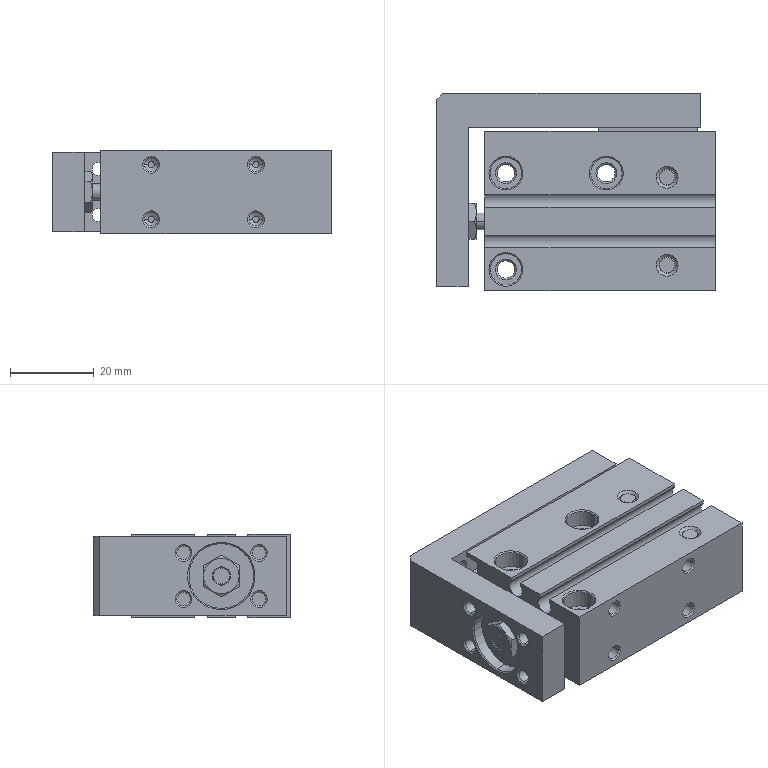Part | STEP file | 2 solids | 358 faces | box 66.5 x 47 x 20 mm | volume 46742 mm3 | cone 130 | cylinder 110 | plane 110 | torus 8 | commonest cylinder face diameters 3.242 x32 4.2 x14 7.5 x12 4.134 x10 0.4 x8 1.74 x8